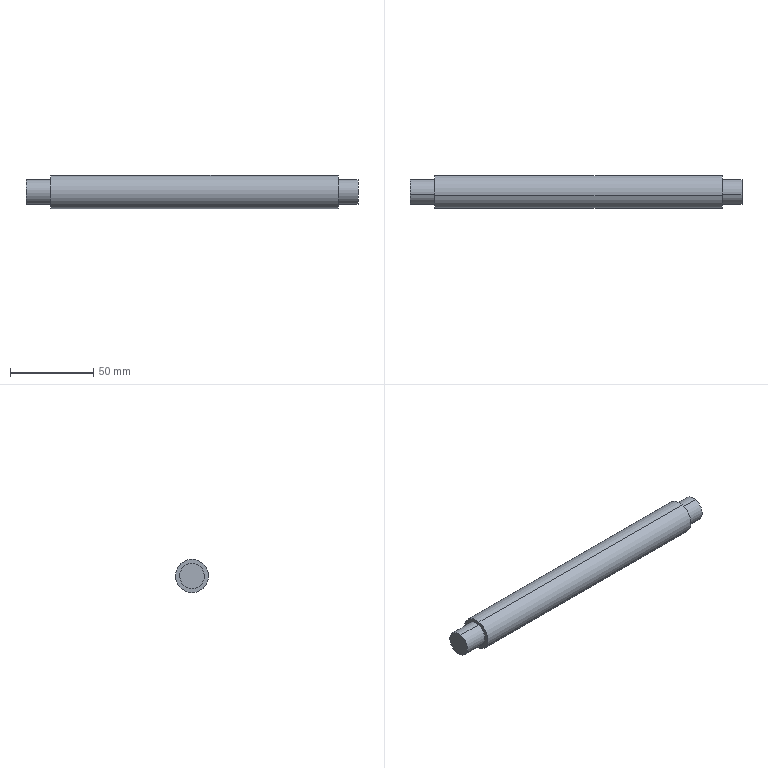Part | SolidWorks | features BaseBody 1 | 1 solid | 10 faces | box 200 x 20 x 20 mm | volume 59121 mm3 | cylinder 6 | plane 4 | commonest cylinder face diameters 15 x4 20 x2
STEP:
#1=CARTESIAN_POINT('',(168.959,74.54,-7.288));
#2=VERTEX_POINT('',#1);
#3=CARTESIAN_POINT('',(168.959,70.997,7.288));
#4=VERTEX_POINT('',#3);
#5=CARTESIAN_POINT('',(168.959,72.768,0.));
#6=DIRECTION('',(-1.,0.,0.));
#7=DIRECTION('',(0.,0.2362,-0.9717));
#8=AXIS2_PLACEMENT_3D('',#5,#6,#7);
#9=CIRCLE('',#8,7.5);
#10=EDGE_CURVE('',#2,#4,#9,.T.);
#11=ORIENTED_EDGE('',*,*,#10,.T.);
#12=CARTESIAN_POINT('',(153.959,70.997,7.288));
#13=VERTEX_POINT('',#12);
#14=CARTESIAN_POINT('',(168.959,70.997,7.288));
#15=DIRECTION('',(-1.,0.,0.));
#16=VECTOR('',#15,1000.);
#17=LINE('',#14,#16);
#18=EDGE_CURVE('',#4,#13,#17,.T.);
#19=ORIENTED_EDGE('',*,*,#18,.T.);
#20=CARTESIAN_POINT('',(153.959,74.54,-7.288));
#21=VERTEX_POINT('',#20);
#22=CARTESIAN_POINT('',(153.959,72.768,0.));
#23=DIRECTION('',(-1.,0.,0.));
#24=DIRECTION('',(0.,0.2362,-0.9717));
#25=AXIS2_PLACEMENT_3D('',#22,#23,#24);
#26=CIRCLE('',#25,7.5);
#27=EDGE_CURVE('',#21,#13,#26,.T.);
#28=ORIENTED_EDGE('',*,*,#27,.F.);
#29=CARTESIAN_POINT('',(168.959,74.54,-7.288));
#30=DIRECTION('',(-1.,0.,0.));
#31=VECTOR('',#30,1000.);
#32=LINE('',#29,#31);
#33=EDGE_CURVE('',#2,#21,#32,.T.);
#34=ORIENTED_EDGE('',*,*,#33,.F.);
#35=EDGE_LOOP('',(#11,#19,#28,#34));
#36=FACE_OUTER_BOUND('',#35,.T.);
#37=CARTESIAN_POINT('',(168.959,72.768,0.));
#38=DIRECTION('',(-1.,0.,0.));
#39=DIRECTION('',(0.,0.2362,-0.9717));
#40=AXIS2_PLACEMENT_3D('',#37,#38,#39);
#41=CYLINDRICAL_SURFACE('',#40,7.5);
#42=ADVANCED_FACE('',(#36),#41,.T.);
#43=CARTESIAN_POINT('',(341.959,70.997,7.288));
#44=VERTEX_POINT('',#43);
#45=CARTESIAN_POINT('',(341.959,74.54,-7.288));
#46=VERTEX_POINT('',#45);
#47=CARTESIAN_POINT('',(341.959,72.768,0.));
#48=DIRECTION('',(1.,0.,0.));
#49=DIRECTION('',(0.,-0.2362,0.9717));
#50=AXIS2_PLACEMENT_3D('',#47,#48,#49);
#51=CIRCLE('',#50,7.5);
#52=EDGE_CURVE('',#44,#46,#51,.T.);
#53=ORIENTED_EDGE('',*,*,#52,.T.);
#54=CARTESIAN_POINT('',(353.959,74.54,-7.288));
#55=VERTEX_POINT('',#54);
#56=CARTESIAN_POINT('',(341.959,74.54,-7.288));
#57=DIRECTION('',(1.,0.,0.));
#58=VECTOR('',#57,1000.);
#59=LINE('',#56,#58);
#60=EDGE_CURVE('',#46,#55,#59,.T.);
#61=ORIENTED_EDGE('',*,*,#60,.T.);
#62=CARTESIAN_POINT('',(353.959,70.997,7.288));
#63=VERTEX_POINT('',#62);
#64=CARTESIAN_POINT('',(353.959,72.768,0.));
#65=DIRECTION('',(1.,0.,0.));
#66=DIRECTION('',(0.,-0.2362,0.9717));
#67=AXIS2_PLACEMENT_3D('',#64,#65,#66);
#68=CIRCLE('',#67,7.5);
#69=EDGE_CURVE('',#63,#55,#68,.T.);
#70=ORIENTED_EDGE('',*,*,#69,.F.);
#71=CARTESIAN_POINT('',(341.959,70.997,7.288));
#72=DIRECTION('',(1.,0.,0.));
#73=VECTOR('',#72,1000.);
#74=LINE('',#71,#73);
#75=EDGE_CURVE('',#44,#63,#74,.T.);
#76=ORIENTED_EDGE('',*,*,#75,.F.);
#77=EDGE_LOOP('',(#53,#61,#70,#76));
#78=FACE_OUTER_BOUND('',#77,.T.);
#79=CARTESIAN_POINT('',(341.959,72.768,0.));
#80=DIRECTION('',(1.,0.,0.));
#81=DIRECTION('',(0.,-0.2362,0.9717));
#82=AXIS2_PLACEMENT_3D('',#79,#80,#81);
#83=CYLINDRICAL_SURFACE('',#82,7.5);
#84=ADVANCED_FACE('',(#78),#83,.T.);
#85=CARTESIAN_POINT('',(341.959,70.407,9.717));
#86=VERTEX_POINT('',#85);
#87=CARTESIAN_POINT('',(341.959,75.13,-9.717));
#88=VERTEX_POINT('',#87);
#89=CARTESIAN_POINT('',(341.959,72.768,0.));
#90=DIRECTION('',(1.,0.,0.));
#91=DIRECTION('',(0.,-0.2362,0.9717));
#92=AXIS2_PLACEMENT_3D('',#89,#90,#91);
#93=CIRCLE('',#92,10.);
#94=EDGE_CURVE('',#86,#88,#93,.T.);
#95=ORIENTED_EDGE('',*,*,#94,.F.);
#96=CARTESIAN_POINT('',(168.959,70.407,9.717));
#97=VERTEX_POINT('',#96);
#98=CARTESIAN_POINT('',(353.959,70.407,9.717));
#99=DIRECTION('',(-1.,0.,0.));
#100=VECTOR('',#99,1000.);
#101=LINE('',#98,#100);
#102=EDGE_CURVE('',#86,#97,#101,.T.);
#103=ORIENTED_EDGE('',*,*,#102,.T.);
#104=CARTESIAN_POINT('',(168.959,75.13,-9.717));
#105=VERTEX_POINT('',#104);
#106=CARTESIAN_POINT('',(168.959,72.768,0.));
#107=DIRECTION('',(-1.,0.,0.));
#108=DIRECTION('',(0.,0.2362,-0.9717));
#109=AXIS2_PLACEMENT_3D('',#106,#107,#108);
#110=CIRCLE('',#109,10.);
#111=EDGE_CURVE('',#105,#97,#110,.T.);
#112=ORIENTED_EDGE('',*,*,#111,.F.);
#113=CARTESIAN_POINT('',(353.959,75.13,-9.717));
#114=DIRECTION('',(-1.,0.,0.));
#115=VECTOR('',#114,1000.);
#116=LINE('',#113,#115);
#117=EDGE_CURVE('',#88,#105,#116,.T.);
#118=ORIENTED_EDGE('',*,*,#117,.F.);
#119=EDGE_LOOP('',(#95,#103,#112,#118));
#120=FACE_OUTER_BOUND('',#119,.T.);
#121=CARTESIAN_POINT('',(353.959,72.768,0.));
#122=DIRECTION('',(-1.,0.,0.));
#123=DIRECTION('',(0.,0.2362,-0.9717));
#124=AXIS2_PLACEMENT_3D('',#121,#122,#123);
#125=CYLINDRICAL_SURFACE('',#124,10.);
#126=ADVANCED_FACE('',(#120),#125,.T.);
#127=ORIENTED_EDGE('',*,*,#102,.F.);
#128=CARTESIAN_POINT('',(341.959,72.768,0.));
#129=DIRECTION('',(1.,0.,0.));
#130=DIRECTION('',(0.,-0.2362,0.9717));
#131=AXIS2_PLACEMENT_3D('',#128,#129,#130);
#132=CIRCLE('',#131,10.);
#133=EDGE_CURVE('',#88,#86,#132,.T.);
#134=ORIENTED_EDGE('',*,*,#133,.F.);
#135=ORIENTED_EDGE('',*,*,#117,.T.);
#136=CARTESIAN_POINT('',(168.959,72.768,0.));
#137=DIRECTION('',(-1.,0.,0.));
#138=DIRECTION('',(0.,0.2362,-0.9717));
#139=AXIS2_PLACEMENT_3D('',#136,#137,#138);
#140=CIRCLE('',#139,10.);
#141=EDGE_CURVE('',#97,#105,#140,.T.);
#142=ORIENTED_EDGE('',*,*,#141,.F.);
#143=EDGE_LOOP('',(#127,#134,#135,#142));
#144=FACE_OUTER_BOUND('',#143,.T.);
#145=CARTESIAN_POINT('',(353.959,72.768,0.));
#146=DIRECTION('',(-1.,0.,0.));
#147=DIRECTION('',(0.,0.2362,-0.9717));
#148=AXIS2_PLACEMENT_3D('',#145,#146,#147);
#149=CYLINDRICAL_SURFACE('',#148,10.);
#150=ADVANCED_FACE('',(#144),#149,.T.);
#151=ORIENTED_EDGE('',*,*,#52,.F.);
#152=CARTESIAN_POINT('',(341.959,72.768,0.));
#153=DIRECTION('',(1.,0.,0.));
#154=DIRECTION('',(0.,-0.2362,0.9717));
#155=AXIS2_PLACEMENT_3D('',#152,#153,#154);
#156=CIRCLE('',#155,7.5);
#157=EDGE_CURVE('',#46,#44,#156,.T.);
#158=ORIENTED_EDGE('',*,*,#157,.F.);
#159=EDGE_LOOP('',(#151,#158));
#160=FACE_BOUND('',#159,.T.);
#161=ORIENTED_EDGE('',*,*,#133,.T.);
#162=ORIENTED_EDGE('',*,*,#94,.T.);
#163=EDGE_LOOP('',(#161,#162));
#164=FACE_OUTER_BOUND('',#163,.T.);
#165=CARTESIAN_POINT('',(341.959,72.768,0.));
#166=DIRECTION('',(1.,0.,0.));
#167=DIRECTION('',(0.,-0.2362,0.9717));
#168=AXIS2_PLACEMENT_3D('',#165,#166,#167);
#169=PLANE('',#168);
#170=ADVANCED_FACE('',(#160,#164),#169,.T.);
#171=ORIENTED_EDGE('',*,*,#60,.F.);
#172=ORIENTED_EDGE('',*,*,#157,.T.);
#173=ORIENTED_EDGE('',*,*,#75,.T.);
#174=CARTESIAN_POINT('',(353.959,72.768,0.));
#175=DIRECTION('',(1.,0.,0.));
#176=DIRECTION('',(0.,-0.2362,0.9717));
#177=AXIS2_PLACEMENT_3D('',#174,#175,#176);
#178=CIRCLE('',#177,7.5);
#179=EDGE_CURVE('',#55,#63,#178,.T.);
#180=ORIENTED_EDGE('',*,*,#179,.F.);
#181=EDGE_LOOP('',(#171,#172,#173,#180));
#182=FACE_OUTER_BOUND('',#181,.T.);
#183=CARTESIAN_POINT('',(341.959,72.768,0.));
#184=DIRECTION('',(1.,0.,0.));
#185=DIRECTION('',(0.,-0.2362,0.9717));
#186=AXIS2_PLACEMENT_3D('',#183,#184,#185);
#187=CYLINDRICAL_SURFACE('',#186,7.5);
#188=ADVANCED_FACE('',(#182),#187,.T.);
#189=ORIENTED_EDGE('',*,*,#69,.T.);
#190=ORIENTED_EDGE('',*,*,#179,.T.);
#191=EDGE_LOOP('',(#189,#190));
#192=FACE_OUTER_BOUND('',#191,.T.);
#193=CARTESIAN_POINT('',(353.959,72.768,0.));
#194=DIRECTION('',(1.,0.,0.));
#195=DIRECTION('',(0.,-0.2362,0.9717));
#196=AXIS2_PLACEMENT_3D('',#193,#194,#195);
#197=PLANE('',#196);
#198=ADVANCED_FACE('',(#192),#197,.T.);
#199=ORIENTED_EDGE('',*,*,#10,.F.);
#200=CARTESIAN_POINT('',(168.959,72.768,0.));
#201=DIRECTION('',(-1.,0.,0.));
#202=DIRECTION('',(0.,0.2362,-0.9717));
#203=AXIS2_PLACEMENT_3D('',#200,#201,#202);
#204=CIRCLE('',#203,7.5);
#205=EDGE_CURVE('',#4,#2,#204,.T.);
#206=ORIENTED_EDGE('',*,*,#205,.F.);
#207=EDGE_LOOP('',(#199,#206));
#208=FACE_BOUND('',#207,.T.);
#209=ORIENTED_EDGE('',*,*,#111,.T.);
#210=ORIENTED_EDGE('',*,*,#141,.T.);
#211=EDGE_LOOP('',(#209,#210));
#212=FACE_OUTER_BOUND('',#211,.T.);
#213=CARTESIAN_POINT('',(168.959,72.768,0.));
#214=DIRECTION('',(-1.,0.,0.));
#215=DIRECTION('',(0.,0.2362,-0.9717));
#216=AXIS2_PLACEMENT_3D('',#213,#214,#215);
#217=PLANE('',#216);
#218=ADVANCED_FACE('',(#208,#212),#217,.T.);
#219=ORIENTED_EDGE('',*,*,#18,.F.);
#220=ORIENTED_EDGE('',*,*,#205,.T.);
#221=ORIENTED_EDGE('',*,*,#33,.T.);
#222=CARTESIAN_POINT('',(153.959,72.768,0.));
#223=DIRECTION('',(-1.,0.,0.));
#224=DIRECTION('',(0.,0.2362,-0.9717));
#225=AXIS2_PLACEMENT_3D('',#222,#223,#224);
#226=CIRCLE('',#225,7.5);
#227=EDGE_CURVE('',#13,#21,#226,.T.);
#228=ORIENTED_EDGE('',*,*,#227,.F.);
#229=EDGE_LOOP('',(#219,#220,#221,#228));
#230=FACE_OUTER_BOUND('',#229,.T.);
#231=CARTESIAN_POINT('',(168.959,72.768,0.));
#232=DIRECTION('',(-1.,0.,0.));
#233=DIRECTION('',(0.,0.2362,-0.9717));
#234=AXIS2_PLACEMENT_3D('',#231,#232,#233);
#235=CYLINDRICAL_SURFACE('',#234,7.5);
#236=ADVANCED_FACE('',(#230),#235,.T.);
#237=ORIENTED_EDGE('',*,*,#27,.T.);
#238=ORIENTED_EDGE('',*,*,#227,.T.);
#239=EDGE_LOOP('',(#237,#238));
#240=FACE_OUTER_BOUND('',#239,.T.);
#241=CARTESIAN_POINT('',(153.959,72.768,0.));
#242=DIRECTION('',(1.,0.,0.));
#243=DIRECTION('',(0.,-0.2362,0.9717));
#244=AXIS2_PLACEMENT_3D('',#241,#242,#243);
#245=PLANE('',#244);
#246=ADVANCED_FACE('',(#240),#245,.F.);
#247=CLOSED_SHELL('',(#42,#84,#126,#150,#170,#188,#198,#218,#236,#246));
#248=MANIFOLD_SOLID_BREP('',#247);
#249=CARTESIAN_POINT('',(0.,0.,0.));
#250=DIRECTION('',(0.,0.,1.));
#251=DIRECTION('',(1.,0.,0.));
#252=AXIS2_PLACEMENT_3D('',#249,#250,#251);
#253=(LENGTH_UNIT()NAMED_UNIT(*)SI_UNIT(.MILLI.,.METRE.));
#254=UNCERTAINTY_MEASURE_WITH_UNIT(LENGTH_MEASURE(0.00001),#253,'','');
#255=(NAMED_UNIT(*)PLANE_ANGLE_UNIT()SI_UNIT($,.RADIAN.));
#256=(NAMED_UNIT(*)SI_UNIT($,.STERADIAN.)SOLID_ANGLE_UNIT());
#257=(GEOMETRIC_REPRESENTATION_CONTEXT(3)GLOBAL_UNCERTAINTY_ASSIGNED_CONTEXT((#254))GLOBAL_UNIT_ASSIGNED_CONTEXT((#253,#255,#256))REPRESENTATION_CONTEXT('',''));
#258=ADVANCED_BREP_SHAPE_REPRESENTATION('',(#248,#252),#257);